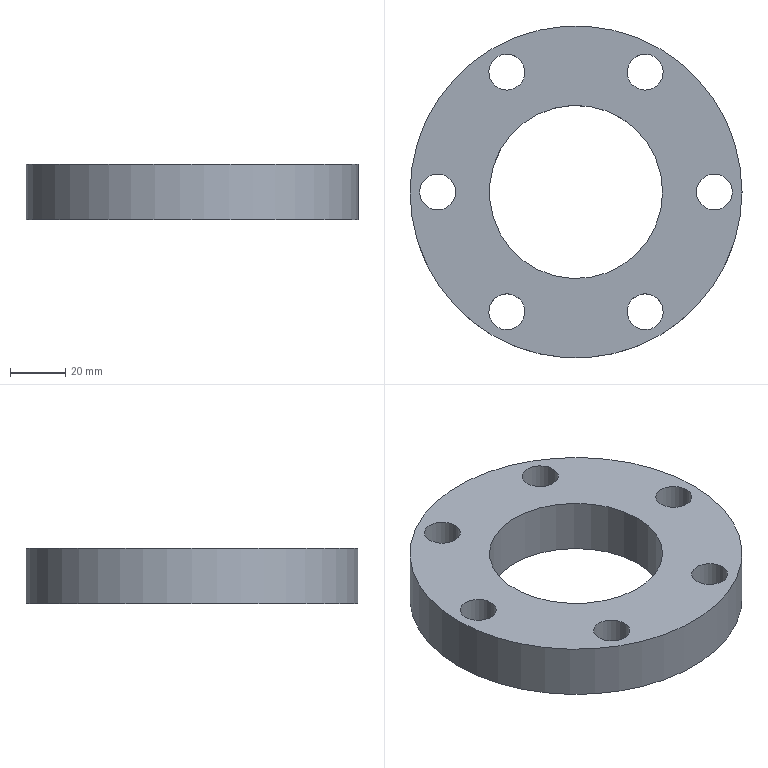NC program | NX | posted with a generic post | part box 120 x 120 x 20 mm
Whole program:
N10 G17 G21 G94 G90
(DRILLING , TOOL : ZXZ)
N12 T01 M6
N14 G54
N16 G17 G0 G90 X25. Y-43.301 S3000 M3
N18 G43 Z70. H1
N20 G94 G81 G98 Z-1. F200. R3.
N22 X-25.
N24 X-50. Y0.
N26 X-25. Y43.301
N28 X25.
N30 X50. Y0.
N32 G80
N34 G0 X50. Y0. Z70.
N36 M5
(DRILLING_COPY , TOOL : 13.0ZT)
N38 T03 M6
N40 G54
N42 G17 G0 G90 X25. Y-43.301 S800 M3
N44 G43 Z70. H3
N46 G94 G83 G98 Z-25.406 F150. Q2. R3.
N48 X-25.
N50 X-50. Y0.
N52 X-25. Y43.301
N54 X25.
N56 X50. Y0.
N58 G80
N60 G0 X50. Y0. Z70.
N62 M5
(ZLEVEL_PROFILE_1_COPY_1 , TOOL : D6A45)
N64 T07 M6
N66 G54
N68 G17 G0 G90 X26.123 Y47.581 S7500 M3
N70 G43 Z70. H7
N72 Z0.
N74 G94 G1 Z-1. F1000.
N76 X25.52 Y48.626
N78 G3 X25. Y48.926 R0.6
N80 X19.376 Y43.301 R5.624
N82 X25. Y48.926 R-5.624
N84 X24.48 Y48.626 R0.6
N86 G1 X23.877 Y47.581
N88 Z0.
N90 G0 Z70.
N92 X-23.877
N94 Z0.
N96 G1 Z-1.
N98 X-24.48 Y48.626
N100 G3 X-25. Y48.926 R0.6
N102 X-30.624 Y43.301 R5.624
N104 X-25. Y48.926 R-5.624
N106 X-25.52 Y48.626 R0.6
N108 G1 X-26.123 Y47.581
N110 Z0.
N112 G0 Z70.
N114 X54.279 Y-1.123
N116 Z0.
N118 G1 Z-1.
N120 X55.324 Y-0.52
N122 G3 X55.624 Y0. R0.6
N124 X50. Y5.624 R5.624
N126 X55.624 Y0. R-5.624
N128 X55.324 Y0.52 R0.6
N130 G1 X54.279 Y1.123
N132 Z0.
N134 G0 Z70.
N136 X-54.279
N138 Z0.
N140 G1 Z-1.
N142 X-55.324 Y0.52
N144 G3 X-55.624 Y0. R0.6
N146 X-50. Y-5.624 R5.624
N148 X-55.624 Y0. R-5.624
N150 X-55.324 Y-0.52 R0.6
N152 G1 X-54.279 Y-1.123
N154 Z0.
N156 G0 Z70.
N158 X23.877 Y-47.581
N160 Z0.
N162 G1 Z-1.
N164 X24.48 Y-48.626
N166 G3 X25. Y-48.926 R0.6
N168 X30.624 Y-43.301 R5.624
N170 X25. Y-48.926 R-5.624
N172 X25.52 Y-48.626 R0.6
N174 G1 X26.123 Y-47.581
N176 Z0.
N178 G0 Z70.
N180 X-26.123
N182 Z0.
N184 G1 Z-1.
N186 X-25.52 Y-48.626
N188 G3 X-25. Y-48.926 R0.6
N190 X-19.376 Y-43.301 R5.624
N192 X-25. Y-48.926 R-5.624
N194 X-24.48 Y-48.626 R0.6
N196 G1 X-23.877 Y-47.581
N198 Z0.
N200 G0 Z70.
N202 M5
N204 M2